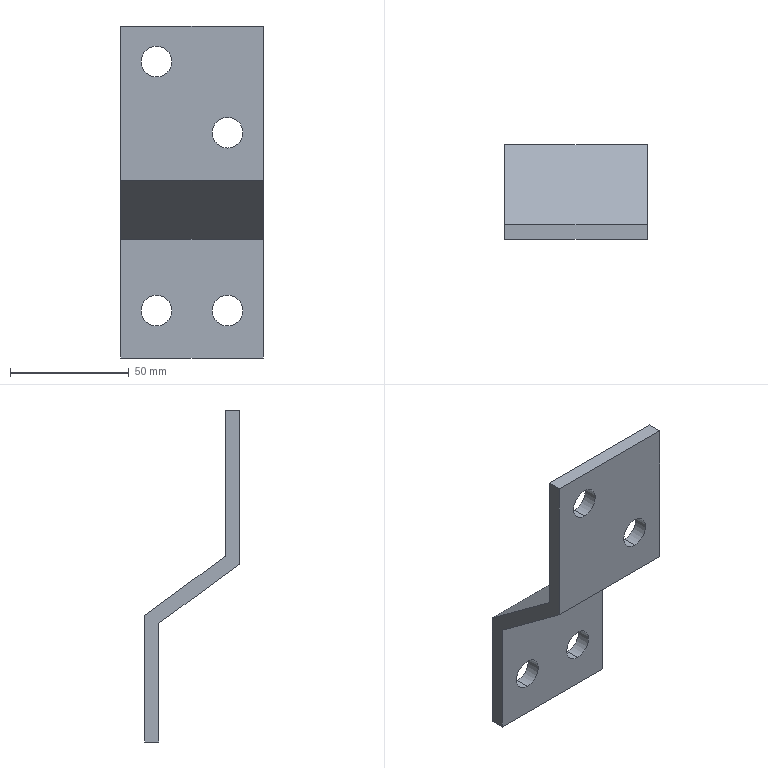Part | SolidWorks | features BaseBody 1 | 1 solid | 18 faces | box 60 x 40 x 140 mm | volume 53998 mm3 | plane 10 | cylinder 8 | commonest cylinder face diameters 13 x8
STEP:
#1=CARTESIAN_POINT('',(741.946,-3252.473,840.471));
#2=VERTEX_POINT('',#1);
#3=CARTESIAN_POINT('',(741.946,-3252.473,827.471));
#4=VERTEX_POINT('',#3);
#5=CARTESIAN_POINT('',(741.946,-3252.473,833.971));
#6=DIRECTION('',(0.,-1.,0.));
#7=DIRECTION('',(0.,0.,-1.));
#8=AXIS2_PLACEMENT_3D('',#5,#6,#7);
#9=CIRCLE('',#8,6.5);
#10=EDGE_CURVE('',#2,#4,#9,.T.);
#11=ORIENTED_EDGE('',*,*,#10,.F.);
#12=CARTESIAN_POINT('',(741.946,-3258.473,840.471));
#13=VERTEX_POINT('',#12);
#14=CARTESIAN_POINT('',(741.946,-3291.307,840.471));
#15=DIRECTION('',(0.,-1.,0.));
#16=VECTOR('',#15,1000.);
#17=LINE('',#14,#16);
#18=EDGE_CURVE('',#2,#13,#17,.T.);
#19=ORIENTED_EDGE('',*,*,#18,.T.);
#20=CARTESIAN_POINT('',(741.946,-3258.473,827.471));
#21=VERTEX_POINT('',#20);
#22=CARTESIAN_POINT('',(741.946,-3258.473,833.971));
#23=DIRECTION('',(0.,1.,0.));
#24=DIRECTION('',(0.,0.,-1.));
#25=AXIS2_PLACEMENT_3D('',#22,#23,#24);
#26=CIRCLE('',#25,6.5);
#27=EDGE_CURVE('',#21,#13,#26,.T.);
#28=ORIENTED_EDGE('',*,*,#27,.F.);
#29=CARTESIAN_POINT('',(741.946,-3291.307,827.471));
#30=DIRECTION('',(0.,-1.,0.));
#31=VECTOR('',#30,1000.);
#32=LINE('',#29,#31);
#33=EDGE_CURVE('',#4,#21,#32,.T.);
#34=ORIENTED_EDGE('',*,*,#33,.F.);
#35=EDGE_LOOP('',(#11,#19,#28,#34));
#36=FACE_OUTER_BOUND('',#35,.T.);
#37=CARTESIAN_POINT('',(741.946,-3291.307,833.971));
#38=DIRECTION('',(0.,-1.,0.));
#39=DIRECTION('',(0.,0.,-1.));
#40=AXIS2_PLACEMENT_3D('',#37,#38,#39);
#41=CYLINDRICAL_SURFACE('',#40,6.5);
#42=ADVANCED_FACE('',(#36),#41,.F.);
#43=CARTESIAN_POINT('',(771.946,-3252.473,810.471));
#44=VERTEX_POINT('',#43);
#45=CARTESIAN_POINT('',(771.946,-3252.473,797.471));
#46=VERTEX_POINT('',#45);
#47=CARTESIAN_POINT('',(771.946,-3252.473,803.971));
#48=DIRECTION('',(0.,-1.,0.));
#49=DIRECTION('',(0.,0.,-1.));
#50=AXIS2_PLACEMENT_3D('',#47,#48,#49);
#51=CIRCLE('',#50,6.5);
#52=EDGE_CURVE('',#44,#46,#51,.T.);
#53=ORIENTED_EDGE('',*,*,#52,.F.);
#54=CARTESIAN_POINT('',(771.946,-3258.473,810.471));
#55=VERTEX_POINT('',#54);
#56=CARTESIAN_POINT('',(771.946,-3246.24,810.471));
#57=DIRECTION('',(0.,-1.,0.));
#58=VECTOR('',#57,1000.);
#59=LINE('',#56,#58);
#60=EDGE_CURVE('',#44,#55,#59,.T.);
#61=ORIENTED_EDGE('',*,*,#60,.T.);
#62=CARTESIAN_POINT('',(771.946,-3258.473,797.471));
#63=VERTEX_POINT('',#62);
#64=CARTESIAN_POINT('',(771.946,-3258.473,803.971));
#65=DIRECTION('',(0.,1.,0.));
#66=DIRECTION('',(0.,0.,-1.));
#67=AXIS2_PLACEMENT_3D('',#64,#65,#66);
#68=CIRCLE('',#67,6.5);
#69=EDGE_CURVE('',#63,#55,#68,.T.);
#70=ORIENTED_EDGE('',*,*,#69,.F.);
#71=CARTESIAN_POINT('',(771.946,-3246.24,797.471));
#72=DIRECTION('',(0.,-1.,0.));
#73=VECTOR('',#72,1000.);
#74=LINE('',#71,#73);
#75=EDGE_CURVE('',#46,#63,#74,.T.);
#76=ORIENTED_EDGE('',*,*,#75,.F.);
#77=EDGE_LOOP('',(#53,#61,#70,#76));
#78=FACE_OUTER_BOUND('',#77,.T.);
#79=CARTESIAN_POINT('',(771.946,-3246.24,803.971));
#80=DIRECTION('',(0.,-1.,0.));
#81=DIRECTION('',(0.,0.,-1.));
#82=AXIS2_PLACEMENT_3D('',#79,#80,#81);
#83=CYLINDRICAL_SURFACE('',#82,6.5);
#84=ADVANCED_FACE('',(#78),#83,.F.);
#85=CARTESIAN_POINT('',(771.946,-3218.473,735.471));
#86=VERTEX_POINT('',#85);
#87=CARTESIAN_POINT('',(771.946,-3218.473,722.471));
#88=VERTEX_POINT('',#87);
#89=CARTESIAN_POINT('',(771.946,-3218.473,728.971));
#90=DIRECTION('',(0.,-1.,0.));
#91=DIRECTION('',(0.,0.,-1.));
#92=AXIS2_PLACEMENT_3D('',#89,#90,#91);
#93=CIRCLE('',#92,6.5);
#94=EDGE_CURVE('',#86,#88,#93,.T.);
#95=ORIENTED_EDGE('',*,*,#94,.F.);
#96=CARTESIAN_POINT('',(771.946,-3224.473,735.471));
#97=VERTEX_POINT('',#96);
#98=CARTESIAN_POINT('',(771.946,-3261.291,735.471));
#99=DIRECTION('',(0.,-1.,0.));
#100=VECTOR('',#99,1000.);
#101=LINE('',#98,#100);
#102=EDGE_CURVE('',#86,#97,#101,.T.);
#103=ORIENTED_EDGE('',*,*,#102,.T.);
#104=CARTESIAN_POINT('',(771.946,-3224.473,722.471));
#105=VERTEX_POINT('',#104);
#106=CARTESIAN_POINT('',(771.946,-3224.473,728.971));
#107=DIRECTION('',(0.,1.,0.));
#108=DIRECTION('',(0.,0.,-1.));
#109=AXIS2_PLACEMENT_3D('',#106,#107,#108);
#110=CIRCLE('',#109,6.5);
#111=EDGE_CURVE('',#105,#97,#110,.T.);
#112=ORIENTED_EDGE('',*,*,#111,.F.);
#113=CARTESIAN_POINT('',(771.946,-3261.291,722.471));
#114=DIRECTION('',(0.,-1.,0.));
#115=VECTOR('',#114,1000.);
#116=LINE('',#113,#115);
#117=EDGE_CURVE('',#88,#105,#116,.T.);
#118=ORIENTED_EDGE('',*,*,#117,.F.);
#119=EDGE_LOOP('',(#95,#103,#112,#118));
#120=FACE_OUTER_BOUND('',#119,.T.);
#121=CARTESIAN_POINT('',(771.946,-3261.291,728.971));
#122=DIRECTION('',(0.,-1.,0.));
#123=DIRECTION('',(0.,0.,-1.));
#124=AXIS2_PLACEMENT_3D('',#121,#122,#123);
#125=CYLINDRICAL_SURFACE('',#124,6.5);
#126=ADVANCED_FACE('',(#120),#125,.F.);
#127=CARTESIAN_POINT('',(741.946,-3218.473,735.471));
#128=VERTEX_POINT('',#127);
#129=CARTESIAN_POINT('',(741.946,-3218.473,722.471));
#130=VERTEX_POINT('',#129);
#131=CARTESIAN_POINT('',(741.946,-3218.473,728.971));
#132=DIRECTION('',(0.,-1.,0.));
#133=DIRECTION('',(0.,0.,-1.));
#134=AXIS2_PLACEMENT_3D('',#131,#132,#133);
#135=CIRCLE('',#134,6.5);
#136=EDGE_CURVE('',#128,#130,#135,.T.);
#137=ORIENTED_EDGE('',*,*,#136,.F.);
#138=CARTESIAN_POINT('',(741.946,-3224.473,735.471));
#139=VERTEX_POINT('',#138);
#140=CARTESIAN_POINT('',(741.946,-3261.291,735.471));
#141=DIRECTION('',(0.,-1.,0.));
#142=VECTOR('',#141,1000.);
#143=LINE('',#140,#142);
#144=EDGE_CURVE('',#128,#139,#143,.T.);
#145=ORIENTED_EDGE('',*,*,#144,.T.);
#146=CARTESIAN_POINT('',(741.946,-3224.473,722.471));
#147=VERTEX_POINT('',#146);
#148=CARTESIAN_POINT('',(741.946,-3224.473,728.971));
#149=DIRECTION('',(0.,1.,0.));
#150=DIRECTION('',(0.,0.,-1.));
#151=AXIS2_PLACEMENT_3D('',#148,#149,#150);
#152=CIRCLE('',#151,6.5);
#153=EDGE_CURVE('',#147,#139,#152,.T.);
#154=ORIENTED_EDGE('',*,*,#153,.F.);
#155=CARTESIAN_POINT('',(741.946,-3261.291,722.471));
#156=DIRECTION('',(0.,-1.,0.));
#157=VECTOR('',#156,1000.);
#158=LINE('',#155,#157);
#159=EDGE_CURVE('',#130,#147,#158,.T.);
#160=ORIENTED_EDGE('',*,*,#159,.F.);
#161=EDGE_LOOP('',(#137,#145,#154,#160));
#162=FACE_OUTER_BOUND('',#161,.T.);
#163=CARTESIAN_POINT('',(741.946,-3261.291,728.971));
#164=DIRECTION('',(0.,-1.,0.));
#165=DIRECTION('',(0.,0.,-1.));
#166=AXIS2_PLACEMENT_3D('',#163,#164,#165);
#167=CYLINDRICAL_SURFACE('',#166,6.5);
#168=ADVANCED_FACE('',(#162),#167,.F.);
#169=CARTESIAN_POINT('',(786.946,-3258.473,783.971));
#170=VERTEX_POINT('',#169);
#171=CARTESIAN_POINT('',(786.946,-3258.473,848.971));
#172=VERTEX_POINT('',#171);
#173=CARTESIAN_POINT('',(786.946,-3258.473,848.971));
#174=DIRECTION('',(0.,0.,1.));
#175=VECTOR('',#174,1000.);
#176=LINE('',#173,#175);
#177=EDGE_CURVE('',#170,#172,#176,.T.);
#178=ORIENTED_EDGE('',*,*,#177,.T.);
#179=CARTESIAN_POINT('',(726.946,-3258.473,848.971));
#180=VERTEX_POINT('',#179);
#181=CARTESIAN_POINT('',(786.946,-3258.473,848.971));
#182=DIRECTION('',(-1.,0.,0.));
#183=VECTOR('',#182,1000.);
#184=LINE('',#181,#183);
#185=EDGE_CURVE('',#172,#180,#184,.T.);
#186=ORIENTED_EDGE('',*,*,#185,.T.);
#187=CARTESIAN_POINT('',(726.946,-3258.473,783.971));
#188=VERTEX_POINT('',#187);
#189=CARTESIAN_POINT('',(726.946,-3258.473,848.971));
#190=DIRECTION('',(0.,0.,-1.));
#191=VECTOR('',#190,1000.);
#192=LINE('',#189,#191);
#193=EDGE_CURVE('',#180,#188,#192,.T.);
#194=ORIENTED_EDGE('',*,*,#193,.T.);
#195=CARTESIAN_POINT('',(786.946,-3258.473,783.971));
#196=DIRECTION('',(1.,0.,0.));
#197=VECTOR('',#196,1000.);
#198=LINE('',#195,#197);
#199=EDGE_CURVE('',#188,#170,#198,.T.);
#200=ORIENTED_EDGE('',*,*,#199,.T.);
#201=EDGE_LOOP('',(#178,#186,#194,#200));
#202=FACE_OUTER_BOUND('',#201,.T.);
#203=ORIENTED_EDGE('',*,*,#27,.T.);
#204=CARTESIAN_POINT('',(741.946,-3258.473,833.971));
#205=DIRECTION('',(0.,1.,0.));
#206=DIRECTION('',(0.,0.,-1.));
#207=AXIS2_PLACEMENT_3D('',#204,#205,#206);
#208=CIRCLE('',#207,6.5);
#209=EDGE_CURVE('',#13,#21,#208,.T.);
#210=ORIENTED_EDGE('',*,*,#209,.T.);
#211=EDGE_LOOP('',(#203,#210));
#212=FACE_BOUND('',#211,.T.);
#213=ORIENTED_EDGE('',*,*,#69,.T.);
#214=CARTESIAN_POINT('',(771.946,-3258.473,803.971));
#215=DIRECTION('',(0.,1.,0.));
#216=DIRECTION('',(0.,0.,-1.));
#217=AXIS2_PLACEMENT_3D('',#214,#215,#216);
#218=CIRCLE('',#217,6.5);
#219=EDGE_CURVE('',#55,#63,#218,.T.);
#220=ORIENTED_EDGE('',*,*,#219,.T.);
#221=EDGE_LOOP('',(#213,#220));
#222=FACE_BOUND('',#221,.T.);
#223=CARTESIAN_POINT('',(786.946,-3258.473,848.971));
#224=DIRECTION('',(0.,-1.,0.));
#225=DIRECTION('',(0.,0.,-1.));
#226=AXIS2_PLACEMENT_3D('',#223,#224,#225);
#227=PLANE('',#226);
#228=ADVANCED_FACE('',(#202,#212,#222),#227,.T.);
#229=CARTESIAN_POINT('',(786.946,-3252.473,848.971));
#230=VERTEX_POINT('',#229);
#231=CARTESIAN_POINT('',(786.946,-3252.473,848.971));
#232=DIRECTION('',(0.,1.,0.));
#233=VECTOR('',#232,1000.);
#234=LINE('',#231,#233);
#235=EDGE_CURVE('',#172,#230,#234,.T.);
#236=ORIENTED_EDGE('',*,*,#235,.T.);
#237=CARTESIAN_POINT('',(726.946,-3252.473,848.971));
#238=VERTEX_POINT('',#237);
#239=CARTESIAN_POINT('',(786.946,-3252.473,848.971));
#240=DIRECTION('',(-1.,0.,0.));
#241=VECTOR('',#240,1000.);
#242=LINE('',#239,#241);
#243=EDGE_CURVE('',#230,#238,#242,.T.);
#244=ORIENTED_EDGE('',*,*,#243,.T.);
#245=CARTESIAN_POINT('',(726.946,-3252.473,848.971));
#246=DIRECTION('',(0.,-1.,0.));
#247=VECTOR('',#246,1000.);
#248=LINE('',#245,#247);
#249=EDGE_CURVE('',#238,#180,#248,.T.);
#250=ORIENTED_EDGE('',*,*,#249,.T.);
#251=ORIENTED_EDGE('',*,*,#185,.F.);
#252=EDGE_LOOP('',(#236,#244,#250,#251));
#253=FACE_OUTER_BOUND('',#252,.T.);
#254=CARTESIAN_POINT('',(786.946,-3252.473,848.971));
#255=DIRECTION('',(0.,0.,1.));
#256=DIRECTION('',(1.,0.,0.));
#257=AXIS2_PLACEMENT_3D('',#254,#255,#256);
#258=PLANE('',#257);
#259=ADVANCED_FACE('',(#253),#258,.T.);
#260=CARTESIAN_POINT('',(786.946,-3224.473,758.971));
#261=VERTEX_POINT('',#260);
#262=CARTESIAN_POINT('',(786.946,-3258.473,783.971));
#263=DIRECTION('',(0.,0.8057,-0.5924));
#264=VECTOR('',#263,1000.);
#265=LINE('',#262,#264);
#266=EDGE_CURVE('',#170,#261,#265,.T.);
#267=ORIENTED_EDGE('',*,*,#266,.T.);
#268=CARTESIAN_POINT('',(786.946,-3224.473,708.971));
#269=VERTEX_POINT('',#268);
#270=CARTESIAN_POINT('',(786.946,-3224.473,778.356));
#271=DIRECTION('',(0.,0.,-1.));
#272=VECTOR('',#271,1000.);
#273=LINE('',#270,#272);
#274=EDGE_CURVE('',#261,#269,#273,.T.);
#275=ORIENTED_EDGE('',*,*,#274,.T.);
#276=CARTESIAN_POINT('',(786.946,-3218.473,708.971));
#277=VERTEX_POINT('',#276);
#278=CARTESIAN_POINT('',(786.946,-3239.689,708.971));
#279=DIRECTION('',(0.,1.,0.));
#280=VECTOR('',#279,1000.);
#281=LINE('',#278,#280);
#282=EDGE_CURVE('',#269,#277,#281,.T.);
#283=ORIENTED_EDGE('',*,*,#282,.T.);
#284=CARTESIAN_POINT('',(786.946,-3218.473,762.297));
#285=VERTEX_POINT('',#284);
#286=CARTESIAN_POINT('',(786.946,-3218.473,778.356));
#287=DIRECTION('',(0.,0.,1.));
#288=VECTOR('',#287,1000.);
#289=LINE('',#286,#288);
#290=EDGE_CURVE('',#277,#285,#289,.T.);
#291=ORIENTED_EDGE('',*,*,#290,.T.);
#292=CARTESIAN_POINT('',(786.946,-3252.473,787.297));
#293=VERTEX_POINT('',#292);
#294=CARTESIAN_POINT('',(786.946,-3218.473,762.297));
#295=DIRECTION('',(0.,-0.8057,0.5924));
#296=VECTOR('',#295,1000.);
#297=LINE('',#294,#296);
#298=EDGE_CURVE('',#285,#293,#297,.T.);
#299=ORIENTED_EDGE('',*,*,#298,.T.);
#300=CARTESIAN_POINT('',(786.946,-3252.473,778.356));
#301=DIRECTION('',(0.,0.,1.));
#302=VECTOR('',#301,1000.);
#303=LINE('',#300,#302);
#304=EDGE_CURVE('',#293,#230,#303,.T.);
#305=ORIENTED_EDGE('',*,*,#304,.T.);
#306=ORIENTED_EDGE('',*,*,#235,.F.);
#307=ORIENTED_EDGE('',*,*,#177,.F.);
#308=EDGE_LOOP('',(#267,#275,#283,#291,#299,#305,#306,#307));
#309=FACE_OUTER_BOUND('',#308,.T.);
#310=CARTESIAN_POINT('',(786.946,-3239.689,778.356));
#311=DIRECTION('',(1.,0.,0.));
#312=DIRECTION('',(0.,0.,-1.));
#313=AXIS2_PLACEMENT_3D('',#310,#311,#312);
#314=PLANE('',#313);
#315=ADVANCED_FACE('',(#309),#314,.T.);
#316=ORIENTED_EDGE('',*,*,#266,.F.);
#317=ORIENTED_EDGE('',*,*,#199,.F.);
#318=CARTESIAN_POINT('',(726.946,-3224.473,758.971));
#319=VERTEX_POINT('',#318);
#320=CARTESIAN_POINT('',(726.946,-3258.473,783.971));
#321=DIRECTION('',(0.,0.8057,-0.5924));
#322=VECTOR('',#321,1000.);
#323=LINE('',#320,#322);
#324=EDGE_CURVE('',#188,#319,#323,.T.);
#325=ORIENTED_EDGE('',*,*,#324,.T.);
#326=CARTESIAN_POINT('',(786.946,-3224.473,758.971));
#327=DIRECTION('',(1.,0.,0.));
#328=VECTOR('',#327,1000.);
#329=LINE('',#326,#328);
#330=EDGE_CURVE('',#319,#261,#329,.T.);
#331=ORIENTED_EDGE('',*,*,#330,.T.);
#332=EDGE_LOOP('',(#316,#317,#325,#331));
#333=FACE_OUTER_BOUND('',#332,.T.);
#334=CARTESIAN_POINT('',(786.946,-3258.473,783.971));
#335=DIRECTION('',(0.,-0.5924,-0.8057));
#336=DIRECTION('',(0.,0.8057,-0.5924));
#337=AXIS2_PLACEMENT_3D('',#334,#335,#336);
#338=PLANE('',#337);
#339=ADVANCED_FACE('',(#333),#338,.T.);
#340=CARTESIAN_POINT('',(726.946,-3224.473,708.971));
#341=VERTEX_POINT('',#340);
#342=CARTESIAN_POINT('',(726.946,-3218.473,708.971));
#343=VERTEX_POINT('',#342);
#344=CARTESIAN_POINT('',(726.946,-3239.689,708.971));
#345=DIRECTION('',(0.,1.,0.));
#346=VECTOR('',#345,1000.);
#347=LINE('',#344,#346);
#348=EDGE_CURVE('',#341,#343,#347,.T.);
#349=ORIENTED_EDGE('',*,*,#348,.F.);
#350=CARTESIAN_POINT('',(726.946,-3224.473,778.356));
#351=DIRECTION('',(0.,0.,-1.));
#352=VECTOR('',#351,1000.);
#353=LINE('',#350,#352);
#354=EDGE_CURVE('',#319,#341,#353,.T.);
#355=ORIENTED_EDGE('',*,*,#354,.F.);
#356=ORIENTED_EDGE('',*,*,#324,.F.);
#357=ORIENTED_EDGE('',*,*,#193,.F.);
#358=ORIENTED_EDGE('',*,*,#249,.F.);
#359=CARTESIAN_POINT('',(726.946,-3252.473,787.297));
#360=VERTEX_POINT('',#359);
#361=CARTESIAN_POINT('',(726.946,-3252.473,778.356));
#362=DIRECTION('',(0.,0.,1.));
#363=VECTOR('',#362,1000.);
#364=LINE('',#361,#363);
#365=EDGE_CURVE('',#360,#238,#364,.T.);
#366=ORIENTED_EDGE('',*,*,#365,.F.);
#367=CARTESIAN_POINT('',(726.946,-3218.473,762.297));
#368=VERTEX_POINT('',#367);
#369=CARTESIAN_POINT('',(726.946,-3218.473,762.297));
#370=DIRECTION('',(0.,-0.8057,0.5924));
#371=VECTOR('',#370,1000.);
#372=LINE('',#369,#371);
#373=EDGE_CURVE('',#368,#360,#372,.T.);
#374=ORIENTED_EDGE('',*,*,#373,.F.);
#375=CARTESIAN_POINT('',(726.946,-3218.473,778.356));
#376=DIRECTION('',(0.,0.,1.));
#377=VECTOR('',#376,1000.);
#378=LINE('',#375,#377);
#379=EDGE_CURVE('',#343,#368,#378,.T.);
#380=ORIENTED_EDGE('',*,*,#379,.F.);
#381=EDGE_LOOP('',(#349,#355,#356,#357,#358,#366,#374,#380));
#382=FACE_OUTER_BOUND('',#381,.T.);
#383=CARTESIAN_POINT('',(726.946,-3239.689,778.356));
#384=DIRECTION('',(1.,0.,0.));
#385=DIRECTION('',(0.,0.,-1.));
#386=AXIS2_PLACEMENT_3D('',#383,#384,#385);
#387=PLANE('',#386);
#388=ADVANCED_FACE('',(#382),#387,.F.);
#389=ORIENTED_EDGE('',*,*,#18,.F.);
#390=CARTESIAN_POINT('',(741.946,-3252.473,833.971));
#391=DIRECTION('',(0.,-1.,0.));
#392=DIRECTION('',(0.,0.,-1.));
#393=AXIS2_PLACEMENT_3D('',#390,#391,#392);
#394=CIRCLE('',#393,6.5);
#395=EDGE_CURVE('',#4,#2,#394,.T.);
#396=ORIENTED_EDGE('',*,*,#395,.F.);
#397=ORIENTED_EDGE('',*,*,#33,.T.);
#398=ORIENTED_EDGE('',*,*,#209,.F.);
#399=EDGE_LOOP('',(#389,#396,#397,#398));
#400=FACE_OUTER_BOUND('',#399,.T.);
#401=CARTESIAN_POINT('',(741.946,-3291.307,833.971));
#402=DIRECTION('',(0.,-1.,0.));
#403=DIRECTION('',(0.,0.,-1.));
#404=AXIS2_PLACEMENT_3D('',#401,#402,#403);
#405=CYLINDRICAL_SURFACE('',#404,6.5);
#406=ADVANCED_FACE('',(#400),#405,.F.);
#407=ORIENTED_EDGE('',*,*,#60,.F.);
#408=CARTESIAN_POINT('',(771.946,-3252.473,803.971));
#409=DIRECTION('',(0.,-1.,0.));
#410=DIRECTION('',(0.,0.,-1.));
#411=AXIS2_PLACEMENT_3D('',#408,#409,#410);
#412=CIRCLE('',#411,6.5);
#413=EDGE_CURVE('',#46,#44,#412,.T.);
#414=ORIENTED_EDGE('',*,*,#413,.F.);
#415=ORIENTED_EDGE('',*,*,#75,.T.);
#416=ORIENTED_EDGE('',*,*,#219,.F.);
#417=EDGE_LOOP('',(#407,#414,#415,#416));
#418=FACE_OUTER_BOUND('',#417,.T.);
#419=CARTESIAN_POINT('',(771.946,-3246.24,803.971));
#420=DIRECTION('',(0.,-1.,0.));
#421=DIRECTION('',(0.,0.,-1.));
#422=AXIS2_PLACEMENT_3D('',#419,#420,#421);
#423=CYLINDRICAL_SURFACE('',#422,6.5);
#424=ADVANCED_FACE('',(#418),#423,.F.);
#425=ORIENTED_EDGE('',*,*,#304,.F.);
#426=CARTESIAN_POINT('',(786.946,-3252.473,787.297));
#427=DIRECTION('',(-1.,0.,0.));
#428=VECTOR('',#427,1000.);
#429=LINE('',#426,#428);
#430=EDGE_CURVE('',#293,#360,#429,.T.);
#431=ORIENTED_EDGE('',*,*,#430,.T.);
#432=ORIENTED_EDGE('',*,*,#365,.T.);
#433=ORIENTED_EDGE('',*,*,#243,.F.);
#434=EDGE_LOOP('',(#425,#431,#432,#433));
#435=FACE_OUTER_BOUND('',#434,.T.);
#436=ORIENTED_EDGE('',*,*,#395,.T.);
#437=ORIENTED_EDGE('',*,*,#10,.T.);
#438=EDGE_LOOP('',(#436,#437));
#439=FACE_BOUND('',#438,.T.);
#440=ORIENTED_EDGE('',*,*,#413,.T.);
#441=ORIENTED_EDGE('',*,*,#52,.T.);
#442=EDGE_LOOP('',(#440,#441));
#443=FACE_BOUND('',#442,.T.);
#444=CARTESIAN_POINT('',(786.946,-3252.473,787.297));
#445=DIRECTION('',(0.,1.,0.));
#446=DIRECTION('',(0.,0.,1.));
#447=AXIS2_PLACEMENT_3D('',#444,#445,#446);
#448=PLANE('',#447);
#449=ADVANCED_FACE('',(#435,#439,#443),#448,.T.);
#450=ORIENTED_EDGE('',*,*,#274,.F.);
#451=ORIENTED_EDGE('',*,*,#330,.F.);
#452=ORIENTED_EDGE('',*,*,#354,.T.);
#453=CARTESIAN_POINT('',(786.946,-3224.473,708.971));
#454=DIRECTION('',(1.,0.,0.));
#455=VECTOR('',#454,1000.);
#456=LINE('',#453,#455);
#457=EDGE_CURVE('',#341,#269,#456,.T.);
#458=ORIENTED_EDGE('',*,*,#457,.T.);
#459=EDGE_LOOP('',(#450,#451,#452,#458));
#460=FACE_OUTER_BOUND('',#459,.T.);
#461=ORIENTED_EDGE('',*,*,#111,.T.);
#462=CARTESIAN_POINT('',(771.946,-3224.473,728.971));
#463=DIRECTION('',(0.,1.,0.));
#464=DIRECTION('',(0.,0.,-1.));
#465=AXIS2_PLACEMENT_3D('',#462,#463,#464);
#466=CIRCLE('',#465,6.5);
#467=EDGE_CURVE('',#97,#105,#466,.T.);
#468=ORIENTED_EDGE('',*,*,#467,.T.);
#469=EDGE_LOOP('',(#461,#468));
#470=FACE_BOUND('',#469,.T.);
#471=ORIENTED_EDGE('',*,*,#153,.T.);
#472=CARTESIAN_POINT('',(741.946,-3224.473,728.971));
#473=DIRECTION('',(0.,1.,0.));
#474=DIRECTION('',(0.,0.,-1.));
#475=AXIS2_PLACEMENT_3D('',#472,#473,#474);
#476=CIRCLE('',#475,6.5);
#477=EDGE_CURVE('',#139,#147,#476,.T.);
#478=ORIENTED_EDGE('',*,*,#477,.T.);
#479=EDGE_LOOP('',(#471,#478));
#480=FACE_BOUND('',#479,.T.);
#481=CARTESIAN_POINT('',(786.946,-3224.473,758.971));
#482=DIRECTION('',(0.,-1.,0.));
#483=DIRECTION('',(0.,0.,-1.));
#484=AXIS2_PLACEMENT_3D('',#481,#482,#483);
#485=PLANE('',#484);
#486=ADVANCED_FACE('',(#460,#470,#480),#485,.T.);
#487=ORIENTED_EDGE('',*,*,#298,.F.);
#488=CARTESIAN_POINT('',(786.946,-3218.473,762.297));
#489=DIRECTION('',(-1.,0.,0.));
#490=VECTOR('',#489,1000.);
#491=LINE('',#488,#490);
#492=EDGE_CURVE('',#285,#368,#491,.T.);
#493=ORIENTED_EDGE('',*,*,#492,.T.);
#494=ORIENTED_EDGE('',*,*,#373,.T.);
#495=ORIENTED_EDGE('',*,*,#430,.F.);
#496=EDGE_LOOP('',(#487,#493,#494,#495));
#497=FACE_OUTER_BOUND('',#496,.T.);
#498=CARTESIAN_POINT('',(786.946,-3218.473,762.297));
#499=DIRECTION('',(0.,0.5924,0.8057));
#500=DIRECTION('',(0.,-0.8057,0.5924));
#501=AXIS2_PLACEMENT_3D('',#498,#499,#500);
#502=PLANE('',#501);
#503=ADVANCED_FACE('',(#497),#502,.T.);
#504=ORIENTED_EDGE('',*,*,#290,.F.);
#505=CARTESIAN_POINT('',(786.946,-3218.473,708.971));
#506=DIRECTION('',(-1.,0.,0.));
#507=VECTOR('',#506,1000.);
#508=LINE('',#505,#507);
#509=EDGE_CURVE('',#277,#343,#508,.T.);
#510=ORIENTED_EDGE('',*,*,#509,.T.);
#511=ORIENTED_EDGE('',*,*,#379,.T.);
#512=ORIENTED_EDGE('',*,*,#492,.F.);
#513=EDGE_LOOP('',(#504,#510,#511,#512));
#514=FACE_OUTER_BOUND('',#513,.T.);
#515=CARTESIAN_POINT('',(771.946,-3218.473,728.971));
#516=DIRECTION('',(0.,-1.,0.));
#517=DIRECTION('',(0.,0.,-1.));
#518=AXIS2_PLACEMENT_3D('',#515,#516,#517);
#519=CIRCLE('',#518,6.5);
#520=EDGE_CURVE('',#88,#86,#519,.T.);
#521=ORIENTED_EDGE('',*,*,#520,.T.);
#522=ORIENTED_EDGE('',*,*,#94,.T.);
#523=EDGE_LOOP('',(#521,#522));
#524=FACE_BOUND('',#523,.T.);
#525=CARTESIAN_POINT('',(741.946,-3218.473,728.971));
#526=DIRECTION('',(0.,-1.,0.));
#527=DIRECTION('',(0.,0.,-1.));
#528=AXIS2_PLACEMENT_3D('',#525,#526,#527);
#529=CIRCLE('',#528,6.5);
#530=EDGE_CURVE('',#130,#128,#529,.T.);
#531=ORIENTED_EDGE('',*,*,#530,.T.);
#532=ORIENTED_EDGE('',*,*,#136,.T.);
#533=EDGE_LOOP('',(#531,#532));
#534=FACE_BOUND('',#533,.T.);
#535=CARTESIAN_POINT('',(786.946,-3218.473,708.971));
#536=DIRECTION('',(0.,1.,0.));
#537=DIRECTION('',(0.,0.,1.));
#538=AXIS2_PLACEMENT_3D('',#535,#536,#537);
#539=PLANE('',#538);
#540=ADVANCED_FACE('',(#514,#524,#534),#539,.T.);
#541=ORIENTED_EDGE('',*,*,#282,.F.);
#542=ORIENTED_EDGE('',*,*,#457,.F.);
#543=ORIENTED_EDGE('',*,*,#348,.T.);
#544=ORIENTED_EDGE('',*,*,#509,.F.);
#545=EDGE_LOOP('',(#541,#542,#543,#544));
#546=FACE_OUTER_BOUND('',#545,.T.);
#547=CARTESIAN_POINT('',(786.946,-3224.473,708.971));
#548=DIRECTION('',(0.,0.,-1.));
#549=DIRECTION('',(-1.,0.,0.));
#550=AXIS2_PLACEMENT_3D('',#547,#548,#549);
#551=PLANE('',#550);
#552=ADVANCED_FACE('',(#546),#551,.T.);
#553=ORIENTED_EDGE('',*,*,#102,.F.);
#554=ORIENTED_EDGE('',*,*,#520,.F.);
#555=ORIENTED_EDGE('',*,*,#117,.T.);
#556=ORIENTED_EDGE('',*,*,#467,.F.);
#557=EDGE_LOOP('',(#553,#554,#555,#556));
#558=FACE_OUTER_BOUND('',#557,.T.);
#559=CARTESIAN_POINT('',(771.946,-3261.291,728.971));
#560=DIRECTION('',(0.,-1.,0.));
#561=DIRECTION('',(0.,0.,-1.));
#562=AXIS2_PLACEMENT_3D('',#559,#560,#561);
#563=CYLINDRICAL_SURFACE('',#562,6.5);
#564=ADVANCED_FACE('',(#558),#563,.F.);
#565=ORIENTED_EDGE('',*,*,#144,.F.);
#566=ORIENTED_EDGE('',*,*,#530,.F.);
#567=ORIENTED_EDGE('',*,*,#159,.T.);
#568=ORIENTED_EDGE('',*,*,#477,.F.);
#569=EDGE_LOOP('',(#565,#566,#567,#568));
#570=FACE_OUTER_BOUND('',#569,.T.);
#571=CARTESIAN_POINT('',(741.946,-3261.291,728.971));
#572=DIRECTION('',(0.,-1.,0.));
#573=DIRECTION('',(0.,0.,-1.));
#574=AXIS2_PLACEMENT_3D('',#571,#572,#573);
#575=CYLINDRICAL_SURFACE('',#574,6.5);
#576=ADVANCED_FACE('',(#570),#575,.F.);
#577=CLOSED_SHELL('',(#42,#84,#126,#168,#228,#259,#315,#339,#388,#406,#424,#449,#486,#503,#540,#552,#564,#576));
#578=MANIFOLD_SOLID_BREP('',#577);
#579=CARTESIAN_POINT('',(0.,0.,0.));
#580=DIRECTION('',(0.,0.,1.));
#581=DIRECTION('',(1.,0.,0.));
#582=AXIS2_PLACEMENT_3D('',#579,#580,#581);
#583=(LENGTH_UNIT()NAMED_UNIT(*)SI_UNIT(.MILLI.,.METRE.));
#584=UNCERTAINTY_MEASURE_WITH_UNIT(LENGTH_MEASURE(0.00001),#583,'','');
#585=(NAMED_UNIT(*)PLANE_ANGLE_UNIT()SI_UNIT($,.RADIAN.));
#586=(NAMED_UNIT(*)SI_UNIT($,.STERADIAN.)SOLID_ANGLE_UNIT());
#587=(GEOMETRIC_REPRESENTATION_CONTEXT(3)GLOBAL_UNCERTAINTY_ASSIGNED_CONTEXT((#584))GLOBAL_UNIT_ASSIGNED_CONTEXT((#583,#585,#586))REPRESENTATION_CONTEXT('',''));
#588=ADVANCED_BREP_SHAPE_REPRESENTATION('',(#578,#582),#587);